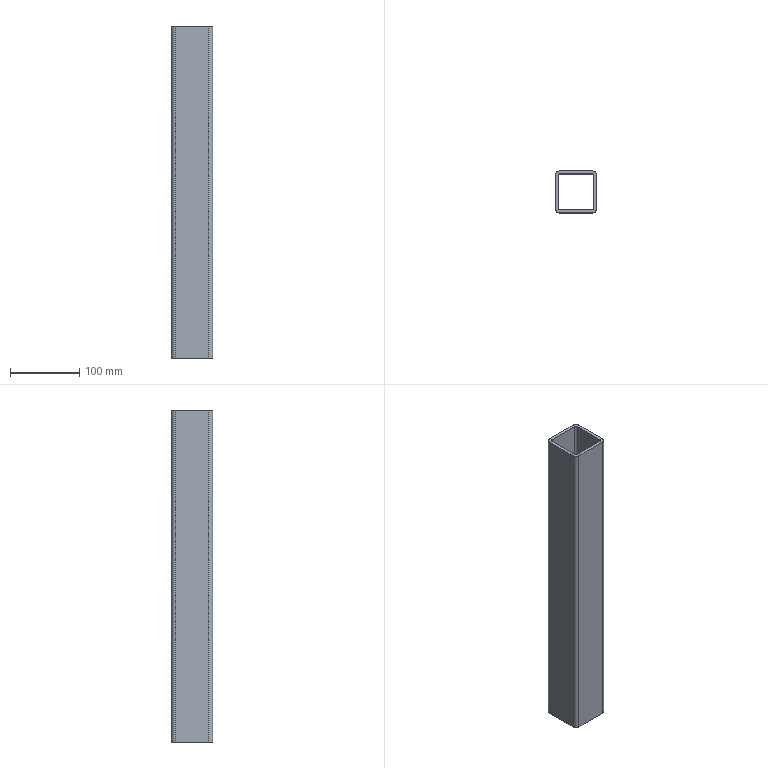Part | SolidWorks | features Fillet 2, Extrusion 1 | 1 solid | 18 faces | box 60 x 60 x 480 mm | volume 418955 mm3 | plane 10 | cylinder 8 | commonest cylinder face diameters 6 x4 12 x4
STEP:
#1=CARTESIAN_POINT('',(-24.,-30.,240.));
#2=VERTEX_POINT('',#1);
#3=CARTESIAN_POINT('',(24.,-30.,240.));
#4=VERTEX_POINT('',#3);
#5=CARTESIAN_POINT('',(-30.,-30.,240.));
#6=DIRECTION('',(1.,0.,0.));
#7=VECTOR('',#6,1000.);
#8=LINE('',#5,#7);
#9=EDGE_CURVE('',#2,#4,#8,.T.);
#10=ORIENTED_EDGE('',*,*,#9,.T.);
#11=CARTESIAN_POINT('',(30.,-24.,240.));
#12=VERTEX_POINT('',#11);
#13=CARTESIAN_POINT('',(24.,-24.,240.));
#14=DIRECTION('',(0.,0.,1.));
#15=DIRECTION('',(-1.,0.,0.));
#16=AXIS2_PLACEMENT_3D('',#13,#14,#15);
#17=CIRCLE('',#16,6.);
#18=EDGE_CURVE('',#4,#12,#17,.T.);
#19=ORIENTED_EDGE('',*,*,#18,.T.);
#20=CARTESIAN_POINT('',(30.,24.,240.));
#21=VERTEX_POINT('',#20);
#22=CARTESIAN_POINT('',(30.,-30.,240.));
#23=DIRECTION('',(0.,1.,0.));
#24=VECTOR('',#23,1000.);
#25=LINE('',#22,#24);
#26=EDGE_CURVE('',#12,#21,#25,.T.);
#27=ORIENTED_EDGE('',*,*,#26,.T.);
#28=CARTESIAN_POINT('',(24.,30.,240.));
#29=VERTEX_POINT('',#28);
#30=CARTESIAN_POINT('',(24.,24.,240.));
#31=DIRECTION('',(0.,0.,1.));
#32=DIRECTION('',(-1.,0.,0.));
#33=AXIS2_PLACEMENT_3D('',#30,#31,#32);
#34=CIRCLE('',#33,6.);
#35=EDGE_CURVE('',#21,#29,#34,.T.);
#36=ORIENTED_EDGE('',*,*,#35,.T.);
#37=CARTESIAN_POINT('',(-24.,30.,240.));
#38=VERTEX_POINT('',#37);
#39=CARTESIAN_POINT('',(-30.,30.,240.));
#40=DIRECTION('',(-1.,0.,0.));
#41=VECTOR('',#40,1000.);
#42=LINE('',#39,#41);
#43=EDGE_CURVE('',#29,#38,#42,.T.);
#44=ORIENTED_EDGE('',*,*,#43,.T.);
#45=CARTESIAN_POINT('',(-30.,24.,240.));
#46=VERTEX_POINT('',#45);
#47=CARTESIAN_POINT('',(-24.,24.,240.));
#48=DIRECTION('',(0.,0.,1.));
#49=DIRECTION('',(-1.,0.,0.));
#50=AXIS2_PLACEMENT_3D('',#47,#48,#49);
#51=CIRCLE('',#50,6.);
#52=EDGE_CURVE('',#38,#46,#51,.T.);
#53=ORIENTED_EDGE('',*,*,#52,.T.);
#54=CARTESIAN_POINT('',(-30.,-24.,240.));
#55=VERTEX_POINT('',#54);
#56=CARTESIAN_POINT('',(-30.,-30.,240.));
#57=DIRECTION('',(0.,-1.,0.));
#58=VECTOR('',#57,1000.);
#59=LINE('',#56,#58);
#60=EDGE_CURVE('',#46,#55,#59,.T.);
#61=ORIENTED_EDGE('',*,*,#60,.T.);
#62=CARTESIAN_POINT('',(-24.,-24.,240.));
#63=DIRECTION('',(0.,0.,1.));
#64=DIRECTION('',(-1.,0.,0.));
#65=AXIS2_PLACEMENT_3D('',#62,#63,#64);
#66=CIRCLE('',#65,6.);
#67=EDGE_CURVE('',#55,#2,#66,.T.);
#68=ORIENTED_EDGE('',*,*,#67,.T.);
#69=EDGE_LOOP('',(#10,#19,#27,#36,#44,#53,#61,#68));
#70=FACE_OUTER_BOUND('',#69,.T.);
#71=CARTESIAN_POINT('',(26.,-23.,240.));
#72=VERTEX_POINT('',#71);
#73=CARTESIAN_POINT('',(26.,23.,240.));
#74=VERTEX_POINT('',#73);
#75=CARTESIAN_POINT('',(26.,-26.,240.));
#76=DIRECTION('',(0.,1.,0.));
#77=VECTOR('',#76,1000.);
#78=LINE('',#75,#77);
#79=EDGE_CURVE('',#72,#74,#78,.T.);
#80=ORIENTED_EDGE('',*,*,#79,.F.);
#81=CARTESIAN_POINT('',(23.,-26.,240.));
#82=VERTEX_POINT('',#81);
#83=CARTESIAN_POINT('',(23.,-23.,240.));
#84=DIRECTION('',(0.,0.,-1.));
#85=DIRECTION('',(-1.,0.,0.));
#86=AXIS2_PLACEMENT_3D('',#83,#84,#85);
#87=CIRCLE('',#86,3.);
#88=EDGE_CURVE('',#72,#82,#87,.T.);
#89=ORIENTED_EDGE('',*,*,#88,.T.);
#90=CARTESIAN_POINT('',(-23.,-26.,240.));
#91=VERTEX_POINT('',#90);
#92=CARTESIAN_POINT('',(-26.,-26.,240.));
#93=DIRECTION('',(1.,0.,0.));
#94=VECTOR('',#93,1000.);
#95=LINE('',#92,#94);
#96=EDGE_CURVE('',#91,#82,#95,.T.);
#97=ORIENTED_EDGE('',*,*,#96,.F.);
#98=CARTESIAN_POINT('',(-26.,-23.,240.));
#99=VERTEX_POINT('',#98);
#100=CARTESIAN_POINT('',(-23.,-23.,240.));
#101=DIRECTION('',(0.,0.,-1.));
#102=DIRECTION('',(-1.,0.,0.));
#103=AXIS2_PLACEMENT_3D('',#100,#101,#102);
#104=CIRCLE('',#103,3.);
#105=EDGE_CURVE('',#91,#99,#104,.T.);
#106=ORIENTED_EDGE('',*,*,#105,.T.);
#107=CARTESIAN_POINT('',(-26.,23.,240.));
#108=VERTEX_POINT('',#107);
#109=CARTESIAN_POINT('',(-26.,-26.,240.));
#110=DIRECTION('',(0.,-1.,0.));
#111=VECTOR('',#110,1000.);
#112=LINE('',#109,#111);
#113=EDGE_CURVE('',#108,#99,#112,.T.);
#114=ORIENTED_EDGE('',*,*,#113,.F.);
#115=CARTESIAN_POINT('',(-23.,26.,240.));
#116=VERTEX_POINT('',#115);
#117=CARTESIAN_POINT('',(-23.,23.,240.));
#118=DIRECTION('',(0.,0.,-1.));
#119=DIRECTION('',(-1.,0.,0.));
#120=AXIS2_PLACEMENT_3D('',#117,#118,#119);
#121=CIRCLE('',#120,3.);
#122=EDGE_CURVE('',#108,#116,#121,.T.);
#123=ORIENTED_EDGE('',*,*,#122,.T.);
#124=CARTESIAN_POINT('',(23.,26.,240.));
#125=VERTEX_POINT('',#124);
#126=CARTESIAN_POINT('',(-26.,26.,240.));
#127=DIRECTION('',(-1.,0.,0.));
#128=VECTOR('',#127,1000.);
#129=LINE('',#126,#128);
#130=EDGE_CURVE('',#125,#116,#129,.T.);
#131=ORIENTED_EDGE('',*,*,#130,.F.);
#132=CARTESIAN_POINT('',(23.,23.,240.));
#133=DIRECTION('',(0.,0.,-1.));
#134=DIRECTION('',(-1.,0.,0.));
#135=AXIS2_PLACEMENT_3D('',#132,#133,#134);
#136=CIRCLE('',#135,3.);
#137=EDGE_CURVE('',#125,#74,#136,.T.);
#138=ORIENTED_EDGE('',*,*,#137,.T.);
#139=EDGE_LOOP('',(#80,#89,#97,#106,#114,#123,#131,#138));
#140=FACE_BOUND('',#139,.T.);
#141=CARTESIAN_POINT('',(0.,0.,240.));
#142=DIRECTION('',(0.,0.,-1.));
#143=DIRECTION('',(-1.,0.,0.));
#144=AXIS2_PLACEMENT_3D('',#141,#142,#143);
#145=PLANE('',#144);
#146=ADVANCED_FACE('',(#70,#140),#145,.F.);
#147=CARTESIAN_POINT('',(30.,-24.,-240.));
#148=VERTEX_POINT('',#147);
#149=CARTESIAN_POINT('',(30.,24.,-240.));
#150=VERTEX_POINT('',#149);
#151=CARTESIAN_POINT('',(30.,-30.,-240.));
#152=DIRECTION('',(0.,1.,0.));
#153=VECTOR('',#152,1000.);
#154=LINE('',#151,#153);
#155=EDGE_CURVE('',#148,#150,#154,.T.);
#156=ORIENTED_EDGE('',*,*,#155,.F.);
#157=CARTESIAN_POINT('',(24.,-30.,-240.));
#158=VERTEX_POINT('',#157);
#159=CARTESIAN_POINT('',(24.,-24.,-240.));
#160=DIRECTION('',(0.,0.,-1.));
#161=DIRECTION('',(-1.,0.,0.));
#162=AXIS2_PLACEMENT_3D('',#159,#160,#161);
#163=CIRCLE('',#162,6.);
#164=EDGE_CURVE('',#148,#158,#163,.T.);
#165=ORIENTED_EDGE('',*,*,#164,.T.);
#166=CARTESIAN_POINT('',(-24.,-30.,-240.));
#167=VERTEX_POINT('',#166);
#168=CARTESIAN_POINT('',(-30.,-30.,-240.));
#169=DIRECTION('',(1.,0.,0.));
#170=VECTOR('',#169,1000.);
#171=LINE('',#168,#170);
#172=EDGE_CURVE('',#167,#158,#171,.T.);
#173=ORIENTED_EDGE('',*,*,#172,.F.);
#174=CARTESIAN_POINT('',(-30.,-24.,-240.));
#175=VERTEX_POINT('',#174);
#176=CARTESIAN_POINT('',(-24.,-24.,-240.));
#177=DIRECTION('',(0.,0.,-1.));
#178=DIRECTION('',(-1.,0.,0.));
#179=AXIS2_PLACEMENT_3D('',#176,#177,#178);
#180=CIRCLE('',#179,6.);
#181=EDGE_CURVE('',#167,#175,#180,.T.);
#182=ORIENTED_EDGE('',*,*,#181,.T.);
#183=CARTESIAN_POINT('',(-30.,24.,-240.));
#184=VERTEX_POINT('',#183);
#185=CARTESIAN_POINT('',(-30.,-30.,-240.));
#186=DIRECTION('',(0.,-1.,0.));
#187=VECTOR('',#186,1000.);
#188=LINE('',#185,#187);
#189=EDGE_CURVE('',#184,#175,#188,.T.);
#190=ORIENTED_EDGE('',*,*,#189,.F.);
#191=CARTESIAN_POINT('',(-24.,30.,-240.));
#192=VERTEX_POINT('',#191);
#193=CARTESIAN_POINT('',(-24.,24.,-240.));
#194=DIRECTION('',(0.,0.,-1.));
#195=DIRECTION('',(-1.,0.,0.));
#196=AXIS2_PLACEMENT_3D('',#193,#194,#195);
#197=CIRCLE('',#196,6.);
#198=EDGE_CURVE('',#184,#192,#197,.T.);
#199=ORIENTED_EDGE('',*,*,#198,.T.);
#200=CARTESIAN_POINT('',(24.,30.,-240.));
#201=VERTEX_POINT('',#200);
#202=CARTESIAN_POINT('',(-30.,30.,-240.));
#203=DIRECTION('',(-1.,0.,0.));
#204=VECTOR('',#203,1000.);
#205=LINE('',#202,#204);
#206=EDGE_CURVE('',#201,#192,#205,.T.);
#207=ORIENTED_EDGE('',*,*,#206,.F.);
#208=CARTESIAN_POINT('',(24.,24.,-240.));
#209=DIRECTION('',(0.,0.,-1.));
#210=DIRECTION('',(-1.,0.,0.));
#211=AXIS2_PLACEMENT_3D('',#208,#209,#210);
#212=CIRCLE('',#211,6.);
#213=EDGE_CURVE('',#201,#150,#212,.T.);
#214=ORIENTED_EDGE('',*,*,#213,.T.);
#215=EDGE_LOOP('',(#156,#165,#173,#182,#190,#199,#207,#214));
#216=FACE_OUTER_BOUND('',#215,.T.);
#217=CARTESIAN_POINT('',(-26.,23.,-240.));
#218=VERTEX_POINT('',#217);
#219=CARTESIAN_POINT('',(-26.,-23.,-240.));
#220=VERTEX_POINT('',#219);
#221=CARTESIAN_POINT('',(-26.,-26.,-240.));
#222=DIRECTION('',(0.,-1.,0.));
#223=VECTOR('',#222,1000.);
#224=LINE('',#221,#223);
#225=EDGE_CURVE('',#218,#220,#224,.T.);
#226=ORIENTED_EDGE('',*,*,#225,.T.);
#227=CARTESIAN_POINT('',(-23.,-26.,-240.));
#228=VERTEX_POINT('',#227);
#229=CARTESIAN_POINT('',(-23.,-23.,-240.));
#230=DIRECTION('',(0.,0.,1.));
#231=DIRECTION('',(-1.,0.,0.));
#232=AXIS2_PLACEMENT_3D('',#229,#230,#231);
#233=CIRCLE('',#232,3.);
#234=EDGE_CURVE('',#220,#228,#233,.T.);
#235=ORIENTED_EDGE('',*,*,#234,.T.);
#236=CARTESIAN_POINT('',(23.,-26.,-240.));
#237=VERTEX_POINT('',#236);
#238=CARTESIAN_POINT('',(-26.,-26.,-240.));
#239=DIRECTION('',(1.,0.,0.));
#240=VECTOR('',#239,1000.);
#241=LINE('',#238,#240);
#242=EDGE_CURVE('',#228,#237,#241,.T.);
#243=ORIENTED_EDGE('',*,*,#242,.T.);
#244=CARTESIAN_POINT('',(26.,-23.,-240.));
#245=VERTEX_POINT('',#244);
#246=CARTESIAN_POINT('',(23.,-23.,-240.));
#247=DIRECTION('',(0.,0.,1.));
#248=DIRECTION('',(-1.,0.,0.));
#249=AXIS2_PLACEMENT_3D('',#246,#247,#248);
#250=CIRCLE('',#249,3.);
#251=EDGE_CURVE('',#237,#245,#250,.T.);
#252=ORIENTED_EDGE('',*,*,#251,.T.);
#253=CARTESIAN_POINT('',(26.,23.,-240.));
#254=VERTEX_POINT('',#253);
#255=CARTESIAN_POINT('',(26.,-26.,-240.));
#256=DIRECTION('',(0.,1.,0.));
#257=VECTOR('',#256,1000.);
#258=LINE('',#255,#257);
#259=EDGE_CURVE('',#245,#254,#258,.T.);
#260=ORIENTED_EDGE('',*,*,#259,.T.);
#261=CARTESIAN_POINT('',(23.,26.,-240.));
#262=VERTEX_POINT('',#261);
#263=CARTESIAN_POINT('',(23.,23.,-240.));
#264=DIRECTION('',(0.,0.,1.));
#265=DIRECTION('',(-1.,0.,0.));
#266=AXIS2_PLACEMENT_3D('',#263,#264,#265);
#267=CIRCLE('',#266,3.);
#268=EDGE_CURVE('',#254,#262,#267,.T.);
#269=ORIENTED_EDGE('',*,*,#268,.T.);
#270=CARTESIAN_POINT('',(-23.,26.,-240.));
#271=VERTEX_POINT('',#270);
#272=CARTESIAN_POINT('',(-26.,26.,-240.));
#273=DIRECTION('',(-1.,0.,0.));
#274=VECTOR('',#273,1000.);
#275=LINE('',#272,#274);
#276=EDGE_CURVE('',#262,#271,#275,.T.);
#277=ORIENTED_EDGE('',*,*,#276,.T.);
#278=CARTESIAN_POINT('',(-23.,23.,-240.));
#279=DIRECTION('',(0.,0.,1.));
#280=DIRECTION('',(-1.,0.,0.));
#281=AXIS2_PLACEMENT_3D('',#278,#279,#280);
#282=CIRCLE('',#281,3.);
#283=EDGE_CURVE('',#271,#218,#282,.T.);
#284=ORIENTED_EDGE('',*,*,#283,.T.);
#285=EDGE_LOOP('',(#226,#235,#243,#252,#260,#269,#277,#284));
#286=FACE_BOUND('',#285,.T.);
#287=CARTESIAN_POINT('',(0.,0.,-240.));
#288=DIRECTION('',(0.,0.,-1.));
#289=DIRECTION('',(-1.,0.,0.));
#290=AXIS2_PLACEMENT_3D('',#287,#288,#289);
#291=PLANE('',#290);
#292=ADVANCED_FACE('',(#216,#286),#291,.T.);
#293=ORIENTED_EDGE('',*,*,#26,.F.);
#294=CARTESIAN_POINT('',(30.,-24.,240.));
#295=DIRECTION('',(0.,0.,-1.));
#296=VECTOR('',#295,1000.);
#297=LINE('',#294,#296);
#298=EDGE_CURVE('',#12,#148,#297,.T.);
#299=ORIENTED_EDGE('',*,*,#298,.T.);
#300=ORIENTED_EDGE('',*,*,#155,.T.);
#301=CARTESIAN_POINT('',(30.,24.,240.));
#302=DIRECTION('',(0.,0.,1.));
#303=VECTOR('',#302,1000.);
#304=LINE('',#301,#303);
#305=EDGE_CURVE('',#150,#21,#304,.T.);
#306=ORIENTED_EDGE('',*,*,#305,.T.);
#307=EDGE_LOOP('',(#293,#299,#300,#306));
#308=FACE_OUTER_BOUND('',#307,.T.);
#309=CARTESIAN_POINT('',(30.,-30.,240.));
#310=DIRECTION('',(-1.,0.,0.));
#311=DIRECTION('',(0.,0.,1.));
#312=AXIS2_PLACEMENT_3D('',#309,#310,#311);
#313=PLANE('',#312);
#314=ADVANCED_FACE('',(#308),#313,.F.);
#315=ORIENTED_EDGE('',*,*,#43,.F.);
#316=CARTESIAN_POINT('',(24.,30.,240.));
#317=DIRECTION('',(0.,0.,-1.));
#318=VECTOR('',#317,1000.);
#319=LINE('',#316,#318);
#320=EDGE_CURVE('',#29,#201,#319,.T.);
#321=ORIENTED_EDGE('',*,*,#320,.T.);
#322=ORIENTED_EDGE('',*,*,#206,.T.);
#323=CARTESIAN_POINT('',(-24.,30.,240.));
#324=DIRECTION('',(0.,0.,1.));
#325=VECTOR('',#324,1000.);
#326=LINE('',#323,#325);
#327=EDGE_CURVE('',#192,#38,#326,.T.);
#328=ORIENTED_EDGE('',*,*,#327,.T.);
#329=EDGE_LOOP('',(#315,#321,#322,#328));
#330=FACE_OUTER_BOUND('',#329,.T.);
#331=CARTESIAN_POINT('',(-30.,30.,240.));
#332=DIRECTION('',(0.,-1.,0.));
#333=DIRECTION('',(0.,0.,-1.));
#334=AXIS2_PLACEMENT_3D('',#331,#332,#333);
#335=PLANE('',#334);
#336=ADVANCED_FACE('',(#330),#335,.F.);
#337=ORIENTED_EDGE('',*,*,#189,.T.);
#338=CARTESIAN_POINT('',(-30.,-24.,240.));
#339=DIRECTION('',(0.,0.,1.));
#340=VECTOR('',#339,1000.);
#341=LINE('',#338,#340);
#342=EDGE_CURVE('',#175,#55,#341,.T.);
#343=ORIENTED_EDGE('',*,*,#342,.T.);
#344=ORIENTED_EDGE('',*,*,#60,.F.);
#345=CARTESIAN_POINT('',(-30.,24.,240.));
#346=DIRECTION('',(0.,0.,-1.));
#347=VECTOR('',#346,1000.);
#348=LINE('',#345,#347);
#349=EDGE_CURVE('',#46,#184,#348,.T.);
#350=ORIENTED_EDGE('',*,*,#349,.T.);
#351=EDGE_LOOP('',(#337,#343,#344,#350));
#352=FACE_OUTER_BOUND('',#351,.T.);
#353=CARTESIAN_POINT('',(-30.,-30.,240.));
#354=DIRECTION('',(1.,0.,0.));
#355=DIRECTION('',(0.,0.,-1.));
#356=AXIS2_PLACEMENT_3D('',#353,#354,#355);
#357=PLANE('',#356);
#358=ADVANCED_FACE('',(#352),#357,.F.);
#359=ORIENTED_EDGE('',*,*,#172,.T.);
#360=CARTESIAN_POINT('',(24.,-30.,240.));
#361=DIRECTION('',(0.,0.,1.));
#362=VECTOR('',#361,1000.);
#363=LINE('',#360,#362);
#364=EDGE_CURVE('',#158,#4,#363,.T.);
#365=ORIENTED_EDGE('',*,*,#364,.T.);
#366=ORIENTED_EDGE('',*,*,#9,.F.);
#367=CARTESIAN_POINT('',(-24.,-30.,240.));
#368=DIRECTION('',(0.,0.,-1.));
#369=VECTOR('',#368,1000.);
#370=LINE('',#367,#369);
#371=EDGE_CURVE('',#2,#167,#370,.T.);
#372=ORIENTED_EDGE('',*,*,#371,.T.);
#373=EDGE_LOOP('',(#359,#365,#366,#372));
#374=FACE_OUTER_BOUND('',#373,.T.);
#375=CARTESIAN_POINT('',(-30.,-30.,240.));
#376=DIRECTION('',(0.,1.,0.));
#377=DIRECTION('',(0.,0.,1.));
#378=AXIS2_PLACEMENT_3D('',#375,#376,#377);
#379=PLANE('',#378);
#380=ADVANCED_FACE('',(#374),#379,.F.);
#381=ORIENTED_EDGE('',*,*,#259,.F.);
#382=CARTESIAN_POINT('',(26.,-23.,240.));
#383=DIRECTION('',(0.,0.,1.));
#384=VECTOR('',#383,1000.);
#385=LINE('',#382,#384);
#386=EDGE_CURVE('',#245,#72,#385,.T.);
#387=ORIENTED_EDGE('',*,*,#386,.T.);
#388=ORIENTED_EDGE('',*,*,#79,.T.);
#389=CARTESIAN_POINT('',(26.,23.,-240.));
#390=DIRECTION('',(0.,0.,-1.));
#391=VECTOR('',#390,1000.);
#392=LINE('',#389,#391);
#393=EDGE_CURVE('',#74,#254,#392,.T.);
#394=ORIENTED_EDGE('',*,*,#393,.T.);
#395=EDGE_LOOP('',(#381,#387,#388,#394));
#396=FACE_OUTER_BOUND('',#395,.T.);
#397=CARTESIAN_POINT('',(26.,-26.,240.));
#398=DIRECTION('',(-1.,0.,0.));
#399=DIRECTION('',(0.,0.,1.));
#400=AXIS2_PLACEMENT_3D('',#397,#398,#399);
#401=PLANE('',#400);
#402=ADVANCED_FACE('',(#396),#401,.T.);
#403=ORIENTED_EDGE('',*,*,#276,.F.);
#404=CARTESIAN_POINT('',(23.,26.,240.));
#405=DIRECTION('',(0.,0.,1.));
#406=VECTOR('',#405,1000.);
#407=LINE('',#404,#406);
#408=EDGE_CURVE('',#262,#125,#407,.T.);
#409=ORIENTED_EDGE('',*,*,#408,.T.);
#410=ORIENTED_EDGE('',*,*,#130,.T.);
#411=CARTESIAN_POINT('',(-23.,26.,-240.));
#412=DIRECTION('',(0.,0.,-1.));
#413=VECTOR('',#412,1000.);
#414=LINE('',#411,#413);
#415=EDGE_CURVE('',#116,#271,#414,.T.);
#416=ORIENTED_EDGE('',*,*,#415,.T.);
#417=EDGE_LOOP('',(#403,#409,#410,#416));
#418=FACE_OUTER_BOUND('',#417,.T.);
#419=CARTESIAN_POINT('',(-26.,26.,240.));
#420=DIRECTION('',(0.,-1.,0.));
#421=DIRECTION('',(0.,0.,-1.));
#422=AXIS2_PLACEMENT_3D('',#419,#420,#421);
#423=PLANE('',#422);
#424=ADVANCED_FACE('',(#418),#423,.T.);
#425=ORIENTED_EDGE('',*,*,#113,.T.);
#426=CARTESIAN_POINT('',(-26.,-23.,-240.));
#427=DIRECTION('',(0.,0.,-1.));
#428=VECTOR('',#427,1000.);
#429=LINE('',#426,#428);
#430=EDGE_CURVE('',#99,#220,#429,.T.);
#431=ORIENTED_EDGE('',*,*,#430,.T.);
#432=ORIENTED_EDGE('',*,*,#225,.F.);
#433=CARTESIAN_POINT('',(-26.,23.,240.));
#434=DIRECTION('',(0.,0.,1.));
#435=VECTOR('',#434,1000.);
#436=LINE('',#433,#435);
#437=EDGE_CURVE('',#218,#108,#436,.T.);
#438=ORIENTED_EDGE('',*,*,#437,.T.);
#439=EDGE_LOOP('',(#425,#431,#432,#438));
#440=FACE_OUTER_BOUND('',#439,.T.);
#441=CARTESIAN_POINT('',(-26.,-26.,240.));
#442=DIRECTION('',(1.,0.,0.));
#443=DIRECTION('',(0.,0.,-1.));
#444=AXIS2_PLACEMENT_3D('',#441,#442,#443);
#445=PLANE('',#444);
#446=ADVANCED_FACE('',(#440),#445,.T.);
#447=ORIENTED_EDGE('',*,*,#96,.T.);
#448=CARTESIAN_POINT('',(23.,-26.,-240.));
#449=DIRECTION('',(0.,0.,-1.));
#450=VECTOR('',#449,1000.);
#451=LINE('',#448,#450);
#452=EDGE_CURVE('',#82,#237,#451,.T.);
#453=ORIENTED_EDGE('',*,*,#452,.T.);
#454=ORIENTED_EDGE('',*,*,#242,.F.);
#455=CARTESIAN_POINT('',(-23.,-26.,240.));
#456=DIRECTION('',(0.,0.,1.));
#457=VECTOR('',#456,1000.);
#458=LINE('',#455,#457);
#459=EDGE_CURVE('',#228,#91,#458,.T.);
#460=ORIENTED_EDGE('',*,*,#459,.T.);
#461=EDGE_LOOP('',(#447,#453,#454,#460));
#462=FACE_OUTER_BOUND('',#461,.T.);
#463=CARTESIAN_POINT('',(-26.,-26.,240.));
#464=DIRECTION('',(0.,1.,0.));
#465=DIRECTION('',(0.,0.,1.));
#466=AXIS2_PLACEMENT_3D('',#463,#464,#465);
#467=PLANE('',#466);
#468=ADVANCED_FACE('',(#462),#467,.T.);
#469=ORIENTED_EDGE('',*,*,#18,.F.);
#470=ORIENTED_EDGE('',*,*,#364,.F.);
#471=ORIENTED_EDGE('',*,*,#164,.F.);
#472=ORIENTED_EDGE('',*,*,#298,.F.);
#473=EDGE_LOOP('',(#469,#470,#471,#472));
#474=FACE_OUTER_BOUND('',#473,.T.);
#475=CARTESIAN_POINT('',(24.,-24.,240.));
#476=DIRECTION('',(0.,0.,-1.));
#477=DIRECTION('',(-1.,0.,0.));
#478=AXIS2_PLACEMENT_3D('',#475,#476,#477);
#479=CYLINDRICAL_SURFACE('',#478,6.);
#480=ADVANCED_FACE('',(#474),#479,.T.);
#481=ORIENTED_EDGE('',*,*,#67,.F.);
#482=ORIENTED_EDGE('',*,*,#342,.F.);
#483=ORIENTED_EDGE('',*,*,#181,.F.);
#484=ORIENTED_EDGE('',*,*,#371,.F.);
#485=EDGE_LOOP('',(#481,#482,#483,#484));
#486=FACE_OUTER_BOUND('',#485,.T.);
#487=CARTESIAN_POINT('',(-24.,-24.,240.));
#488=DIRECTION('',(0.,0.,-1.));
#489=DIRECTION('',(-1.,0.,0.));
#490=AXIS2_PLACEMENT_3D('',#487,#488,#489);
#491=CYLINDRICAL_SURFACE('',#490,6.);
#492=ADVANCED_FACE('',(#486),#491,.T.);
#493=ORIENTED_EDGE('',*,*,#35,.F.);
#494=ORIENTED_EDGE('',*,*,#305,.F.);
#495=ORIENTED_EDGE('',*,*,#213,.F.);
#496=ORIENTED_EDGE('',*,*,#320,.F.);
#497=EDGE_LOOP('',(#493,#494,#495,#496));
#498=FACE_OUTER_BOUND('',#497,.T.);
#499=CARTESIAN_POINT('',(24.,24.,240.));
#500=DIRECTION('',(0.,0.,-1.));
#501=DIRECTION('',(-1.,0.,0.));
#502=AXIS2_PLACEMENT_3D('',#499,#500,#501);
#503=CYLINDRICAL_SURFACE('',#502,6.);
#504=ADVANCED_FACE('',(#498),#503,.T.);
#505=ORIENTED_EDGE('',*,*,#52,.F.);
#506=ORIENTED_EDGE('',*,*,#327,.F.);
#507=ORIENTED_EDGE('',*,*,#198,.F.);
#508=ORIENTED_EDGE('',*,*,#349,.F.);
#509=EDGE_LOOP('',(#505,#506,#507,#508));
#510=FACE_OUTER_BOUND('',#509,.T.);
#511=CARTESIAN_POINT('',(-24.,24.,240.));
#512=DIRECTION('',(0.,0.,-1.));
#513=DIRECTION('',(-1.,0.,0.));
#514=AXIS2_PLACEMENT_3D('',#511,#512,#513);
#515=CYLINDRICAL_SURFACE('',#514,6.);
#516=ADVANCED_FACE('',(#510),#515,.T.);
#517=ORIENTED_EDGE('',*,*,#88,.F.);
#518=ORIENTED_EDGE('',*,*,#386,.F.);
#519=ORIENTED_EDGE('',*,*,#251,.F.);
#520=ORIENTED_EDGE('',*,*,#452,.F.);
#521=EDGE_LOOP('',(#517,#518,#519,#520));
#522=FACE_OUTER_BOUND('',#521,.T.);
#523=CARTESIAN_POINT('',(23.,-23.,240.));
#524=DIRECTION('',(0.,0.,1.));
#525=DIRECTION('',(1.,0.,0.));
#526=AXIS2_PLACEMENT_3D('',#523,#524,#525);
#527=CYLINDRICAL_SURFACE('',#526,3.);
#528=ADVANCED_FACE('',(#522),#527,.F.);
#529=ORIENTED_EDGE('',*,*,#105,.F.);
#530=ORIENTED_EDGE('',*,*,#459,.F.);
#531=ORIENTED_EDGE('',*,*,#234,.F.);
#532=ORIENTED_EDGE('',*,*,#430,.F.);
#533=EDGE_LOOP('',(#529,#530,#531,#532));
#534=FACE_OUTER_BOUND('',#533,.T.);
#535=CARTESIAN_POINT('',(-23.,-23.,240.));
#536=DIRECTION('',(0.,0.,1.));
#537=DIRECTION('',(1.,0.,0.));
#538=AXIS2_PLACEMENT_3D('',#535,#536,#537);
#539=CYLINDRICAL_SURFACE('',#538,3.);
#540=ADVANCED_FACE('',(#534),#539,.F.);
#541=ORIENTED_EDGE('',*,*,#137,.F.);
#542=ORIENTED_EDGE('',*,*,#408,.F.);
#543=ORIENTED_EDGE('',*,*,#268,.F.);
#544=ORIENTED_EDGE('',*,*,#393,.F.);
#545=EDGE_LOOP('',(#541,#542,#543,#544));
#546=FACE_OUTER_BOUND('',#545,.T.);
#547=CARTESIAN_POINT('',(23.,23.,240.));
#548=DIRECTION('',(0.,0.,1.));
#549=DIRECTION('',(1.,0.,0.));
#550=AXIS2_PLACEMENT_3D('',#547,#548,#549);
#551=CYLINDRICAL_SURFACE('',#550,3.);
#552=ADVANCED_FACE('',(#546),#551,.F.);
#553=ORIENTED_EDGE('',*,*,#122,.F.);
#554=ORIENTED_EDGE('',*,*,#437,.F.);
#555=ORIENTED_EDGE('',*,*,#283,.F.);
#556=ORIENTED_EDGE('',*,*,#415,.F.);
#557=EDGE_LOOP('',(#553,#554,#555,#556));
#558=FACE_OUTER_BOUND('',#557,.T.);
#559=CARTESIAN_POINT('',(-23.,23.,240.));
#560=DIRECTION('',(0.,0.,1.));
#561=DIRECTION('',(1.,0.,0.));
#562=AXIS2_PLACEMENT_3D('',#559,#560,#561);
#563=CYLINDRICAL_SURFACE('',#562,3.);
#564=ADVANCED_FACE('',(#558),#563,.F.);
#565=CLOSED_SHELL('',(#146,#292,#314,#336,#358,#380,#402,#424,#446,#468,#480,#492,#504,#516,#528,#540,#552,#564));
#566=MANIFOLD_SOLID_BREP('',#565);
#567=CARTESIAN_POINT('',(0.,0.,0.));
#568=DIRECTION('',(0.,0.,1.));
#569=DIRECTION('',(1.,0.,0.));
#570=AXIS2_PLACEMENT_3D('',#567,#568,#569);
#571=(LENGTH_UNIT()NAMED_UNIT(*)SI_UNIT(.MILLI.,.METRE.));
#572=UNCERTAINTY_MEASURE_WITH_UNIT(LENGTH_MEASURE(0.00001),#571,'','');
#573=(NAMED_UNIT(*)PLANE_ANGLE_UNIT()SI_UNIT($,.RADIAN.));
#574=(NAMED_UNIT(*)SI_UNIT($,.STERADIAN.)SOLID_ANGLE_UNIT());
#575=(GEOMETRIC_REPRESENTATION_CONTEXT(3)GLOBAL_UNCERTAINTY_ASSIGNED_CONTEXT((#572))GLOBAL_UNIT_ASSIGNED_CONTEXT((#571,#573,#574))REPRESENTATION_CONTEXT('',''));
#576=ADVANCED_BREP_SHAPE_REPRESENTATION('',(#566,#570),#575);